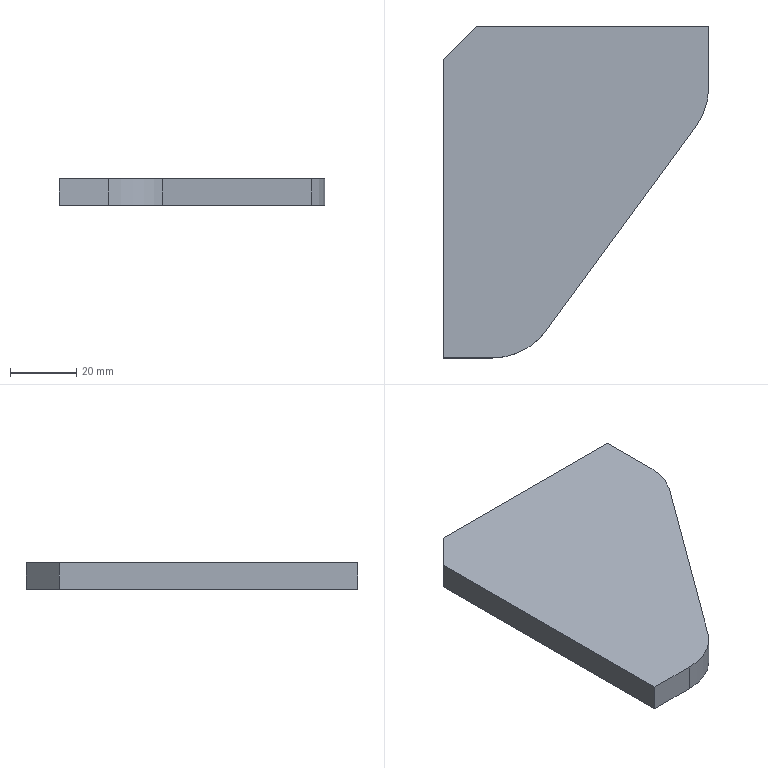Part | SolidWorks | features BaseBody 1 | 1 solid | 10 faces | box 80 x 100 x 8 mm | volume 46944 mm3 | plane 8 | cylinder 2 | commonest cylinder face diameters 40 x2
STEP:
#1=CARTESIAN_POINT('',(-40.,-50.,-4.));
#2=VERTEX_POINT('',#1);
#3=CARTESIAN_POINT('',(-25.135,-50.,-4.));
#4=VERTEX_POINT('',#3);
#5=CARTESIAN_POINT('',(-40.,-50.,-4.));
#6=DIRECTION('',(1.,0.,0.));
#7=VECTOR('',#6,1000.);
#8=LINE('',#5,#7);
#9=EDGE_CURVE('',#2,#4,#8,.T.);
#10=ORIENTED_EDGE('',*,*,#9,.T.);
#11=CARTESIAN_POINT('',(-25.135,-50.,4.));
#12=VERTEX_POINT('',#11);
#13=CARTESIAN_POINT('',(-25.135,-50.,4.));
#14=DIRECTION('',(0.,0.,-1.));
#15=VECTOR('',#14,1000.);
#16=LINE('',#13,#15);
#17=EDGE_CURVE('',#12,#4,#16,.T.);
#18=ORIENTED_EDGE('',*,*,#17,.F.);
#19=CARTESIAN_POINT('',(-40.,-50.,4.));
#20=VERTEX_POINT('',#19);
#21=CARTESIAN_POINT('',(-40.,-50.,4.));
#22=DIRECTION('',(1.,0.,0.));
#23=VECTOR('',#22,1000.);
#24=LINE('',#21,#23);
#25=EDGE_CURVE('',#20,#12,#24,.T.);
#26=ORIENTED_EDGE('',*,*,#25,.F.);
#27=CARTESIAN_POINT('',(-40.,-50.,4.));
#28=DIRECTION('',(0.,0.,-1.));
#29=VECTOR('',#28,1000.);
#30=LINE('',#27,#29);
#31=EDGE_CURVE('',#20,#2,#30,.T.);
#32=ORIENTED_EDGE('',*,*,#31,.T.);
#33=EDGE_LOOP('',(#10,#18,#26,#32));
#34=FACE_OUTER_BOUND('',#33,.T.);
#35=CARTESIAN_POINT('',(-40.,-50.,4.));
#36=DIRECTION('',(0.,1.,0.));
#37=DIRECTION('',(0.,0.,1.));
#38=AXIS2_PLACEMENT_3D('',#35,#36,#37);
#39=PLANE('',#38);
#40=ADVANCED_FACE('',(#34),#39,.F.);
#41=CARTESIAN_POINT('',(-9.007,-41.827,-4.));
#42=VERTEX_POINT('',#41);
#43=CARTESIAN_POINT('',(-25.135,-30.,-4.));
#44=DIRECTION('',(0.,0.,1.));
#45=DIRECTION('',(-1.,0.,0.));
#46=AXIS2_PLACEMENT_3D('',#43,#44,#45);
#47=CIRCLE('',#46,20.);
#48=EDGE_CURVE('',#4,#42,#47,.T.);
#49=ORIENTED_EDGE('',*,*,#48,.T.);
#50=CARTESIAN_POINT('',(-9.007,-41.827,4.));
#51=VERTEX_POINT('',#50);
#52=CARTESIAN_POINT('',(-9.007,-41.827,4.));
#53=DIRECTION('',(0.,0.,-1.));
#54=VECTOR('',#53,1000.);
#55=LINE('',#52,#54);
#56=EDGE_CURVE('',#51,#42,#55,.T.);
#57=ORIENTED_EDGE('',*,*,#56,.F.);
#58=CARTESIAN_POINT('',(-25.135,-30.,4.));
#59=DIRECTION('',(0.,0.,1.));
#60=DIRECTION('',(-1.,0.,0.));
#61=AXIS2_PLACEMENT_3D('',#58,#59,#60);
#62=CIRCLE('',#61,20.);
#63=EDGE_CURVE('',#12,#51,#62,.T.);
#64=ORIENTED_EDGE('',*,*,#63,.F.);
#65=ORIENTED_EDGE('',*,*,#17,.T.);
#66=EDGE_LOOP('',(#49,#57,#64,#65));
#67=FACE_OUTER_BOUND('',#66,.T.);
#68=CARTESIAN_POINT('',(-25.135,-30.,4.));
#69=DIRECTION('',(0.,0.,-1.));
#70=DIRECTION('',(-1.,0.,0.));
#71=AXIS2_PLACEMENT_3D('',#68,#69,#70);
#72=CYLINDRICAL_SURFACE('',#71,20.);
#73=ADVANCED_FACE('',(#67),#72,.T.);
#74=CARTESIAN_POINT('',(36.128,19.72,-4.));
#75=VERTEX_POINT('',#74);
#76=CARTESIAN_POINT('',(36.128,19.72,-4.));
#77=DIRECTION('',(0.5914,0.8064,0.));
#78=VECTOR('',#77,1000.);
#79=LINE('',#76,#78);
#80=EDGE_CURVE('',#42,#75,#79,.T.);
#81=ORIENTED_EDGE('',*,*,#80,.T.);
#82=CARTESIAN_POINT('',(36.128,19.72,4.));
#83=VERTEX_POINT('',#82);
#84=CARTESIAN_POINT('',(36.128,19.72,4.));
#85=DIRECTION('',(0.,0.,-1.));
#86=VECTOR('',#85,1000.);
#87=LINE('',#84,#86);
#88=EDGE_CURVE('',#83,#75,#87,.T.);
#89=ORIENTED_EDGE('',*,*,#88,.F.);
#90=CARTESIAN_POINT('',(36.128,19.72,4.));
#91=DIRECTION('',(0.5914,0.8064,0.));
#92=VECTOR('',#91,1000.);
#93=LINE('',#90,#92);
#94=EDGE_CURVE('',#51,#83,#93,.T.);
#95=ORIENTED_EDGE('',*,*,#94,.F.);
#96=ORIENTED_EDGE('',*,*,#56,.T.);
#97=EDGE_LOOP('',(#81,#89,#95,#96));
#98=FACE_OUTER_BOUND('',#97,.T.);
#99=CARTESIAN_POINT('',(36.128,19.72,4.));
#100=DIRECTION('',(-0.8064,0.5914,0.));
#101=DIRECTION('',(-0.5914,-0.8064,0.));
#102=AXIS2_PLACEMENT_3D('',#99,#100,#101);
#103=PLANE('',#102);
#104=ADVANCED_FACE('',(#98),#103,.F.);
#105=CARTESIAN_POINT('',(40.,31.547,-4.));
#106=VERTEX_POINT('',#105);
#107=CARTESIAN_POINT('',(20.,31.547,-4.));
#108=DIRECTION('',(0.,0.,1.));
#109=DIRECTION('',(1.,0.,0.));
#110=AXIS2_PLACEMENT_3D('',#107,#108,#109);
#111=CIRCLE('',#110,20.);
#112=EDGE_CURVE('',#75,#106,#111,.T.);
#113=ORIENTED_EDGE('',*,*,#112,.T.);
#114=CARTESIAN_POINT('',(40.,31.547,4.));
#115=VERTEX_POINT('',#114);
#116=CARTESIAN_POINT('',(40.,31.547,4.));
#117=DIRECTION('',(0.,0.,-1.));
#118=VECTOR('',#117,1000.);
#119=LINE('',#116,#118);
#120=EDGE_CURVE('',#115,#106,#119,.T.);
#121=ORIENTED_EDGE('',*,*,#120,.F.);
#122=CARTESIAN_POINT('',(20.,31.547,4.));
#123=DIRECTION('',(0.,0.,1.));
#124=DIRECTION('',(1.,0.,0.));
#125=AXIS2_PLACEMENT_3D('',#122,#123,#124);
#126=CIRCLE('',#125,20.);
#127=EDGE_CURVE('',#83,#115,#126,.T.);
#128=ORIENTED_EDGE('',*,*,#127,.F.);
#129=ORIENTED_EDGE('',*,*,#88,.T.);
#130=EDGE_LOOP('',(#113,#121,#128,#129));
#131=FACE_OUTER_BOUND('',#130,.T.);
#132=CARTESIAN_POINT('',(20.,31.547,4.));
#133=DIRECTION('',(0.,0.,-1.));
#134=DIRECTION('',(-1.,0.,0.));
#135=AXIS2_PLACEMENT_3D('',#132,#133,#134);
#136=CYLINDRICAL_SURFACE('',#135,20.);
#137=ADVANCED_FACE('',(#131),#136,.T.);
#138=CARTESIAN_POINT('',(40.,50.,-4.));
#139=VERTEX_POINT('',#138);
#140=CARTESIAN_POINT('',(40.,50.,-4.));
#141=DIRECTION('',(0.,1.,0.));
#142=VECTOR('',#141,1000.);
#143=LINE('',#140,#142);
#144=EDGE_CURVE('',#106,#139,#143,.T.);
#145=ORIENTED_EDGE('',*,*,#144,.T.);
#146=CARTESIAN_POINT('',(40.,50.,4.));
#147=VERTEX_POINT('',#146);
#148=CARTESIAN_POINT('',(40.,50.,4.));
#149=DIRECTION('',(0.,0.,-1.));
#150=VECTOR('',#149,1000.);
#151=LINE('',#148,#150);
#152=EDGE_CURVE('',#147,#139,#151,.T.);
#153=ORIENTED_EDGE('',*,*,#152,.F.);
#154=CARTESIAN_POINT('',(40.,50.,4.));
#155=DIRECTION('',(0.,1.,0.));
#156=VECTOR('',#155,1000.);
#157=LINE('',#154,#156);
#158=EDGE_CURVE('',#115,#147,#157,.T.);
#159=ORIENTED_EDGE('',*,*,#158,.F.);
#160=ORIENTED_EDGE('',*,*,#120,.T.);
#161=EDGE_LOOP('',(#145,#153,#159,#160));
#162=FACE_OUTER_BOUND('',#161,.T.);
#163=CARTESIAN_POINT('',(40.,50.,4.));
#164=DIRECTION('',(-1.,0.,0.));
#165=DIRECTION('',(0.,0.,1.));
#166=AXIS2_PLACEMENT_3D('',#163,#164,#165);
#167=PLANE('',#166);
#168=ADVANCED_FACE('',(#162),#167,.F.);
#169=CARTESIAN_POINT('',(-30.,50.,-4.));
#170=VERTEX_POINT('',#169);
#171=CARTESIAN_POINT('',(-30.,50.,-4.));
#172=DIRECTION('',(-1.,0.,0.));
#173=VECTOR('',#172,1000.);
#174=LINE('',#171,#173);
#175=EDGE_CURVE('',#139,#170,#174,.T.);
#176=ORIENTED_EDGE('',*,*,#175,.T.);
#177=CARTESIAN_POINT('',(-30.,50.,4.));
#178=VERTEX_POINT('',#177);
#179=CARTESIAN_POINT('',(-30.,50.,4.));
#180=DIRECTION('',(0.,0.,-1.));
#181=VECTOR('',#180,1000.);
#182=LINE('',#179,#181);
#183=EDGE_CURVE('',#178,#170,#182,.T.);
#184=ORIENTED_EDGE('',*,*,#183,.F.);
#185=CARTESIAN_POINT('',(-30.,50.,4.));
#186=DIRECTION('',(-1.,0.,0.));
#187=VECTOR('',#186,1000.);
#188=LINE('',#185,#187);
#189=EDGE_CURVE('',#147,#178,#188,.T.);
#190=ORIENTED_EDGE('',*,*,#189,.F.);
#191=ORIENTED_EDGE('',*,*,#152,.T.);
#192=EDGE_LOOP('',(#176,#184,#190,#191));
#193=FACE_OUTER_BOUND('',#192,.T.);
#194=CARTESIAN_POINT('',(-30.,50.,4.));
#195=DIRECTION('',(0.,-1.,0.));
#196=DIRECTION('',(0.,0.,-1.));
#197=AXIS2_PLACEMENT_3D('',#194,#195,#196);
#198=PLANE('',#197);
#199=ADVANCED_FACE('',(#193),#198,.F.);
#200=CARTESIAN_POINT('',(-40.,40.,-4.));
#201=VERTEX_POINT('',#200);
#202=CARTESIAN_POINT('',(-40.,40.,-4.));
#203=DIRECTION('',(-0.7071,-0.7071,0.));
#204=VECTOR('',#203,1000.);
#205=LINE('',#202,#204);
#206=EDGE_CURVE('',#170,#201,#205,.T.);
#207=ORIENTED_EDGE('',*,*,#206,.T.);
#208=CARTESIAN_POINT('',(-40.,40.,4.));
#209=VERTEX_POINT('',#208);
#210=CARTESIAN_POINT('',(-40.,40.,4.));
#211=DIRECTION('',(0.,0.,-1.));
#212=VECTOR('',#211,1000.);
#213=LINE('',#210,#212);
#214=EDGE_CURVE('',#209,#201,#213,.T.);
#215=ORIENTED_EDGE('',*,*,#214,.F.);
#216=CARTESIAN_POINT('',(-40.,40.,4.));
#217=DIRECTION('',(-0.7071,-0.7071,0.));
#218=VECTOR('',#217,1000.);
#219=LINE('',#216,#218);
#220=EDGE_CURVE('',#178,#209,#219,.T.);
#221=ORIENTED_EDGE('',*,*,#220,.F.);
#222=ORIENTED_EDGE('',*,*,#183,.T.);
#223=EDGE_LOOP('',(#207,#215,#221,#222));
#224=FACE_OUTER_BOUND('',#223,.T.);
#225=CARTESIAN_POINT('',(-40.,40.,4.));
#226=DIRECTION('',(0.7071,-0.7071,0.));
#227=DIRECTION('',(0.7071,0.7071,0.));
#228=AXIS2_PLACEMENT_3D('',#225,#226,#227);
#229=PLANE('',#228);
#230=ADVANCED_FACE('',(#224),#229,.F.);
#231=CARTESIAN_POINT('',(-40.,40.,-4.));
#232=DIRECTION('',(0.,-1.,0.));
#233=VECTOR('',#232,1000.);
#234=LINE('',#231,#233);
#235=EDGE_CURVE('',#201,#2,#234,.T.);
#236=ORIENTED_EDGE('',*,*,#235,.T.);
#237=ORIENTED_EDGE('',*,*,#31,.F.);
#238=CARTESIAN_POINT('',(-40.,40.,4.));
#239=DIRECTION('',(0.,-1.,0.));
#240=VECTOR('',#239,1000.);
#241=LINE('',#238,#240);
#242=EDGE_CURVE('',#209,#20,#241,.T.);
#243=ORIENTED_EDGE('',*,*,#242,.F.);
#244=ORIENTED_EDGE('',*,*,#214,.T.);
#245=EDGE_LOOP('',(#236,#237,#243,#244));
#246=FACE_OUTER_BOUND('',#245,.T.);
#247=CARTESIAN_POINT('',(-40.,40.,4.));
#248=DIRECTION('',(1.,0.,0.));
#249=DIRECTION('',(0.,1.,0.));
#250=AXIS2_PLACEMENT_3D('',#247,#248,#249);
#251=PLANE('',#250);
#252=ADVANCED_FACE('',(#246),#251,.F.);
#253=ORIENTED_EDGE('',*,*,#25,.T.);
#254=ORIENTED_EDGE('',*,*,#63,.T.);
#255=ORIENTED_EDGE('',*,*,#94,.T.);
#256=ORIENTED_EDGE('',*,*,#127,.T.);
#257=ORIENTED_EDGE('',*,*,#158,.T.);
#258=ORIENTED_EDGE('',*,*,#189,.T.);
#259=ORIENTED_EDGE('',*,*,#220,.T.);
#260=ORIENTED_EDGE('',*,*,#242,.T.);
#261=EDGE_LOOP('',(#253,#254,#255,#256,#257,#258,#259,#260));
#262=FACE_OUTER_BOUND('',#261,.T.);
#263=CARTESIAN_POINT('',(-25.135,-30.,4.));
#264=DIRECTION('',(0.,0.,-1.));
#265=DIRECTION('',(-1.,0.,0.));
#266=AXIS2_PLACEMENT_3D('',#263,#264,#265);
#267=PLANE('',#266);
#268=ADVANCED_FACE('',(#262),#267,.F.);
#269=ORIENTED_EDGE('',*,*,#9,.F.);
#270=ORIENTED_EDGE('',*,*,#235,.F.);
#271=ORIENTED_EDGE('',*,*,#206,.F.);
#272=ORIENTED_EDGE('',*,*,#175,.F.);
#273=ORIENTED_EDGE('',*,*,#144,.F.);
#274=ORIENTED_EDGE('',*,*,#112,.F.);
#275=ORIENTED_EDGE('',*,*,#80,.F.);
#276=ORIENTED_EDGE('',*,*,#48,.F.);
#277=EDGE_LOOP('',(#269,#270,#271,#272,#273,#274,#275,#276));
#278=FACE_OUTER_BOUND('',#277,.T.);
#279=CARTESIAN_POINT('',(-25.135,-30.,-4.));
#280=DIRECTION('',(0.,0.,-1.));
#281=DIRECTION('',(-1.,0.,0.));
#282=AXIS2_PLACEMENT_3D('',#279,#280,#281);
#283=PLANE('',#282);
#284=ADVANCED_FACE('',(#278),#283,.T.);
#285=CLOSED_SHELL('',(#40,#73,#104,#137,#168,#199,#230,#252,#268,#284));
#286=MANIFOLD_SOLID_BREP('',#285);
#287=CARTESIAN_POINT('',(0.,0.,0.));
#288=DIRECTION('',(0.,0.,1.));
#289=DIRECTION('',(1.,0.,0.));
#290=AXIS2_PLACEMENT_3D('',#287,#288,#289);
#291=(LENGTH_UNIT()NAMED_UNIT(*)SI_UNIT(.MILLI.,.METRE.));
#292=UNCERTAINTY_MEASURE_WITH_UNIT(LENGTH_MEASURE(0.00001),#291,'','');
#293=(NAMED_UNIT(*)PLANE_ANGLE_UNIT()SI_UNIT($,.RADIAN.));
#294=(NAMED_UNIT(*)SI_UNIT($,.STERADIAN.)SOLID_ANGLE_UNIT());
#295=(GEOMETRIC_REPRESENTATION_CONTEXT(3)GLOBAL_UNCERTAINTY_ASSIGNED_CONTEXT((#292))GLOBAL_UNIT_ASSIGNED_CONTEXT((#291,#293,#294))REPRESENTATION_CONTEXT('',''));
#296=ADVANCED_BREP_SHAPE_REPRESENTATION('',(#286,#290),#295);